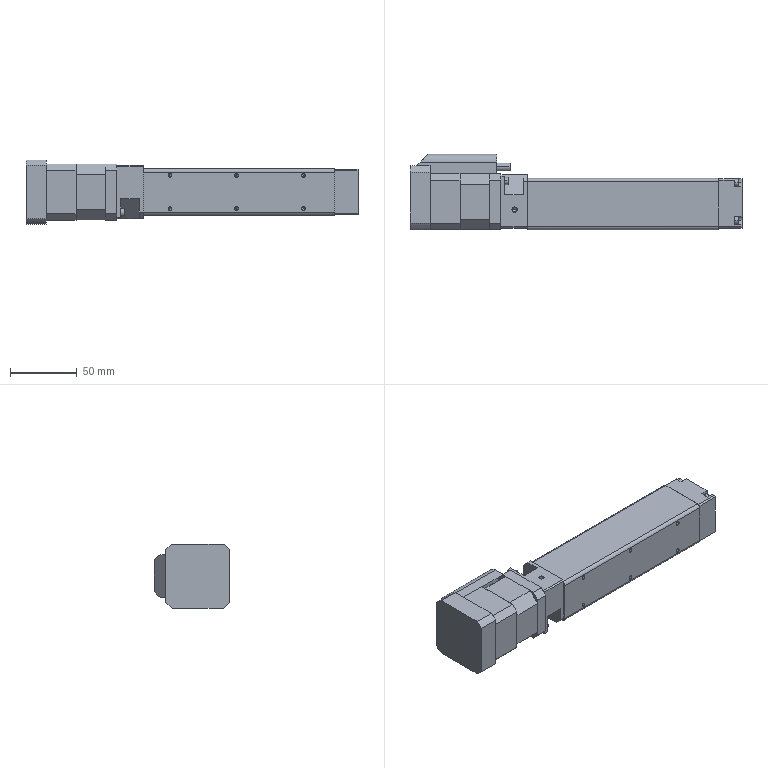Part | STEP file | Guide wheel mechanism revised.sldasm-Part-421 | 1 solid | 233 faces | box 249 x 56.5 x 48 mm | volume 376427 mm3 | plane 110 | cone 64 | cylinder 59 | commonest cylinder face diameters 2.459 x20 5.5 x12 6 x9 3.242 x6 5 x4 57.9 x4